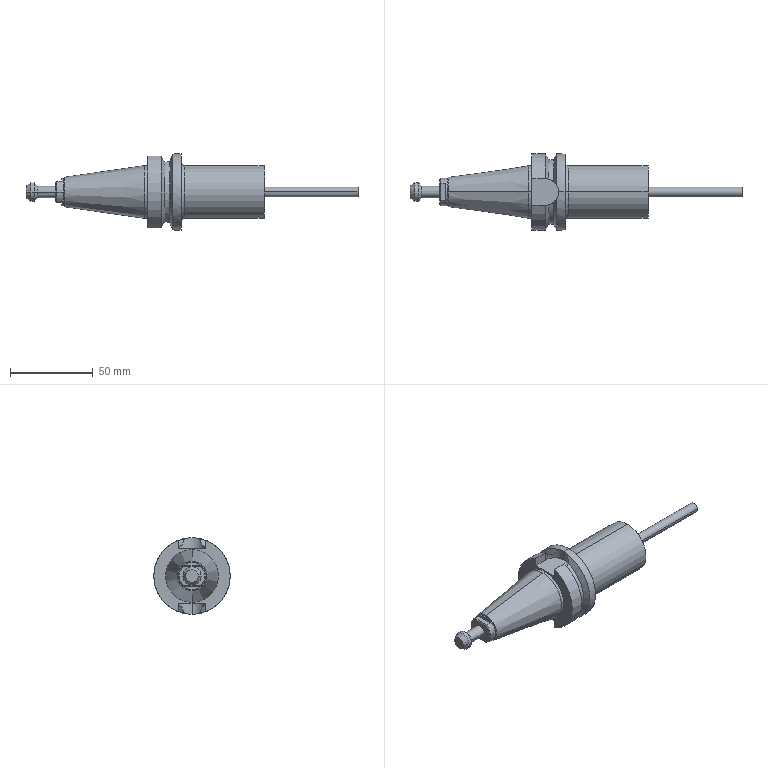Part | SolidWorks | features BaseBody 10, MoveFace 1 | 10 solids | 141 faces | box 200 x 46 x 46 mm | volume 92799 mm3 | plane 53 | cylinder 51 | cone 29 | torus 8 | commonest cylinder face diameters 3 x6 21 x6 6 x4 12 x4 46 x4 16.1 x3